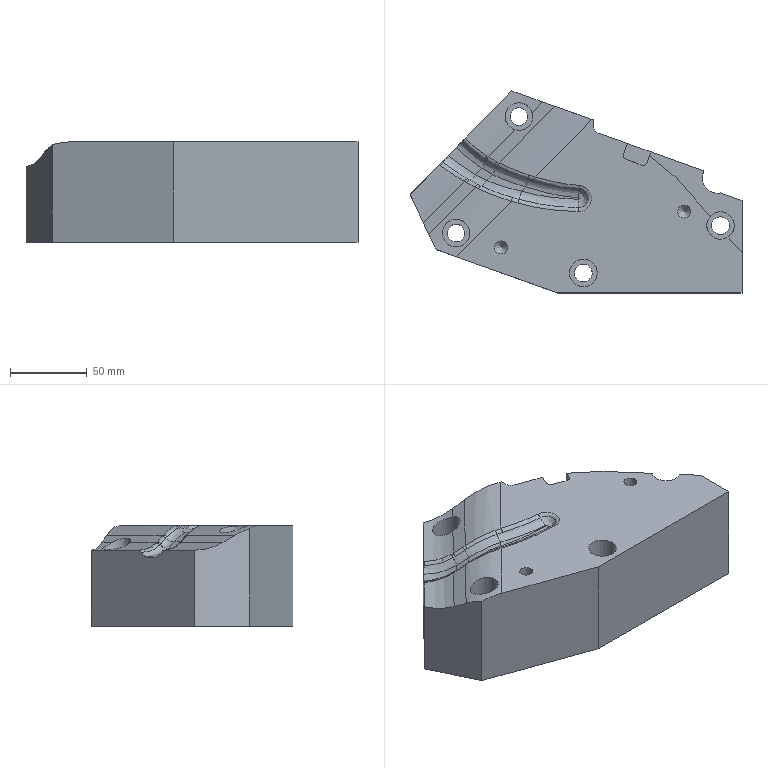Part | NX | features 23 2 | 1 solid | 99 faces | box 216.494 x 131.72 x 65.4 mm | volume 1131904 mm3 | plane 36 | cylinder 29 | spline 25 | torus 5 | cone 4 | commonest cylinder face diameters 15 x6 18 x5 11.5 x4 4.3 x2 6 x2 8.5 x2